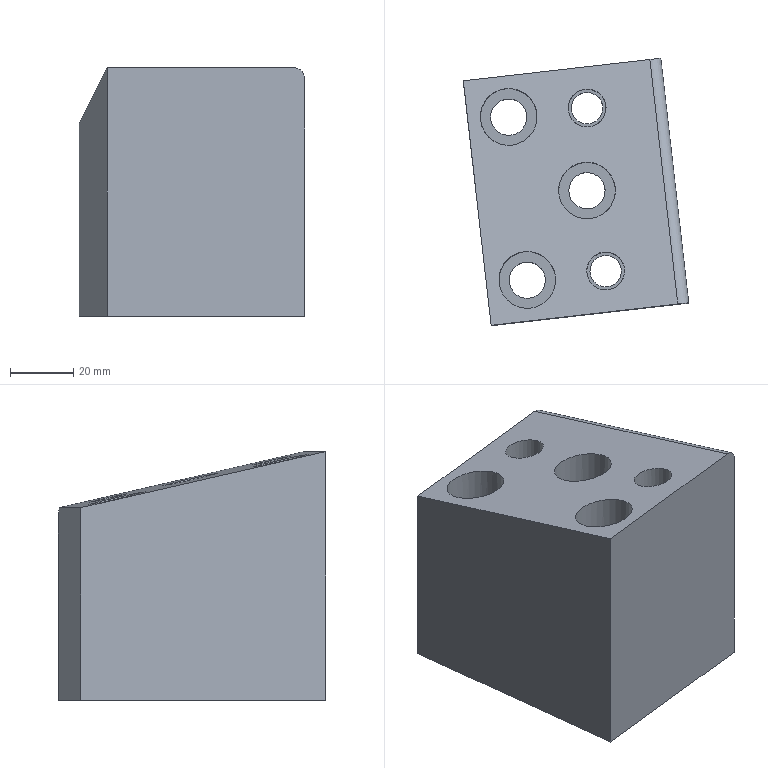Part | NX | features 23 2 | 1 solid | 22 faces | box 71.425 x 84.63 x 78.868 mm | volume 289986 mm3 | plane 11 | cylinder 11 | commonest cylinder face diameters 11.5 x3 18 x3 10.001 x2 12 x2 7 x1
STEP:
#1=CARTESIAN_POINT('',(3732.12,240.405,-83.));
#2=VERTEX_POINT('',#1);
#3=CARTESIAN_POINT('',(3726.517,239.111,-83.));
#4=DIRECTION('',(0.,0.,1.));
#5=DIRECTION('',(0.9744,0.225,0.));
#6=AXIS2_PLACEMENT_3D('',#3,#4,#5);
#7=CIRCLE('',#6,5.75);
#8=EDGE_CURVE('',#2,#2,#7,.T.);
#9=ORIENTED_EDGE('',*,*,#8,.F.);
#10=EDGE_LOOP('',(#9));
#11=FACE_BOUND('',#10,.T.);
#12=CARTESIAN_POINT('',(3735.286,241.136,-83.));
#13=VERTEX_POINT('',#12);
#14=CARTESIAN_POINT('',(3726.517,239.111,-83.));
#15=DIRECTION('',(0.,0.,1.));
#16=DIRECTION('',(0.9744,0.225,0.));
#17=AXIS2_PLACEMENT_3D('',#14,#15,#16);
#18=CIRCLE('',#17,9.);
#19=EDGE_CURVE('',#13,#13,#18,.T.);
#20=ORIENTED_EDGE('',*,*,#19,.T.);
#21=EDGE_LOOP('',(#20));
#22=FACE_BOUND('',#21,.T.);
#23=CARTESIAN_POINT('',(3726.517,239.111,-83.));
#24=DIRECTION('',(0.,0.,-1.));
#25=DIRECTION('',(-0.9744,-0.225,0.));
#26=AXIS2_PLACEMENT_3D('',#23,#24,#25);
#27=PLANE('',#26);
#28=ADVANCED_FACE('',(#11,#22),#27,.F.);
#29=CARTESIAN_POINT('',(3720.767,239.111,-113.));
#30=VERTEX_POINT('',#29);
#31=CARTESIAN_POINT('',(3726.517,239.111,-113.));
#32=DIRECTION('',(0.,0.,1.));
#33=DIRECTION('',(-1.,0.,0.));
#34=AXIS2_PLACEMENT_3D('',#31,#32,#33);
#35=CIRCLE('',#34,5.75);
#36=EDGE_CURVE('',#30,#30,#35,.T.);
#37=ORIENTED_EDGE('',*,*,#36,.F.);
#38=EDGE_LOOP('',(#37));
#39=FACE_BOUND('',#38,.T.);
#40=ORIENTED_EDGE('',*,*,#8,.T.);
#41=EDGE_LOOP('',(#40));
#42=FACE_BOUND('',#41,.T.);
#43=CARTESIAN_POINT('',(3726.517,239.111,-9.166));
#44=DIRECTION('',(0.,0.,-1.));
#45=DIRECTION('',(-0.9744,-0.225,0.));
#46=AXIS2_PLACEMENT_3D('',#43,#44,#45);
#47=CYLINDRICAL_SURFACE('',#46,5.75);
#48=ADVANCED_FACE('',(#39,#42),#47,.F.);
#49=CARTESIAN_POINT('',(3725.498,248.054,-39.145));
#50=VERTEX_POINT('',#49);
#51=CARTESIAN_POINT('',(3726.517,239.111,-37.094));
#52=DIRECTION('',(-0.02515,0.2207,0.975));
#53=DIRECTION('',(-0.1104,0.9687,-0.2221));
#54=AXIS2_PLACEMENT_3D('',#51,#52,#53);
#55=ELLIPSE('',#54,9.231,9.);
#56=EDGE_CURVE('',#50,#50,#55,.T.);
#57=ORIENTED_EDGE('',*,*,#56,.T.);
#58=EDGE_LOOP('',(#57));
#59=FACE_BOUND('',#58,.T.);
#60=ORIENTED_EDGE('',*,*,#19,.F.);
#61=EDGE_LOOP('',(#60));
#62=FACE_BOUND('',#61,.T.);
#63=CARTESIAN_POINT('',(3726.517,239.111,-34.166));
#64=DIRECTION('',(0.,0.,-1.));
#65=DIRECTION('',(-0.9744,-0.225,0.));
#66=AXIS2_PLACEMENT_3D('',#63,#64,#65);
#67=CYLINDRICAL_SURFACE('',#66,9.);
#68=ADVANCED_FACE('',(#59,#62),#67,.F.);
#69=CARTESIAN_POINT('',(3751.035,268.728,-83.));
#70=VERTEX_POINT('',#69);
#71=CARTESIAN_POINT('',(3745.432,267.435,-83.));
#72=DIRECTION('',(0.,0.,1.));
#73=DIRECTION('',(0.9744,0.225,0.));
#74=AXIS2_PLACEMENT_3D('',#71,#72,#73);
#75=CIRCLE('',#74,5.75);
#76=EDGE_CURVE('',#70,#70,#75,.T.);
#77=ORIENTED_EDGE('',*,*,#76,.F.);
#78=EDGE_LOOP('',(#77));
#79=FACE_BOUND('',#78,.T.);
#80=CARTESIAN_POINT('',(3754.202,269.459,-83.));
#81=VERTEX_POINT('',#80);
#82=CARTESIAN_POINT('',(3745.432,267.435,-83.));
#83=DIRECTION('',(0.,0.,1.));
#84=DIRECTION('',(0.9744,0.225,0.));
#85=AXIS2_PLACEMENT_3D('',#82,#83,#84);
#86=CIRCLE('',#85,9.);
#87=EDGE_CURVE('',#81,#81,#86,.T.);
#88=ORIENTED_EDGE('',*,*,#87,.T.);
#89=EDGE_LOOP('',(#88));
#90=FACE_BOUND('',#89,.T.);
#91=CARTESIAN_POINT('',(3745.416,267.58,-83.));
#92=DIRECTION('',(0.,0.,-1.));
#93=DIRECTION('',(-0.9744,-0.225,0.));
#94=AXIS2_PLACEMENT_3D('',#91,#92,#93);
#95=PLANE('',#94);
#96=ADVANCED_FACE('',(#79,#90),#95,.F.);
#97=CARTESIAN_POINT('',(3756.357,241.942,-84.));
#98=VERTEX_POINT('',#97);
#99=CARTESIAN_POINT('',(3751.356,241.942,-84.));
#100=DIRECTION('',(0.,0.,1.));
#101=DIRECTION('',(1.,0.,0.));
#102=AXIS2_PLACEMENT_3D('',#99,#100,#101);
#103=CIRCLE('',#102,5.);
#104=EDGE_CURVE('',#98,#98,#103,.T.);
#105=ORIENTED_EDGE('',*,*,#104,.F.);
#106=EDGE_LOOP('',(#105));
#107=FACE_BOUND('',#106,.T.);
#108=CARTESIAN_POINT('',(3757.356,241.942,-84.));
#109=VERTEX_POINT('',#108);
#110=CARTESIAN_POINT('',(3751.356,241.942,-84.));
#111=DIRECTION('',(0.,0.,1.));
#112=DIRECTION('',(1.,0.,0.));
#113=AXIS2_PLACEMENT_3D('',#110,#111,#112);
#114=CIRCLE('',#113,6.);
#115=EDGE_CURVE('',#109,#109,#114,.T.);
#116=ORIENTED_EDGE('',*,*,#115,.T.);
#117=EDGE_LOOP('',(#116));
#118=FACE_BOUND('',#117,.T.);
#119=CARTESIAN_POINT('',(3751.34,242.086,-84.));
#120=DIRECTION('',(0.,0.,-1.));
#121=DIRECTION('',(-1.,0.,0.));
#122=AXIS2_PLACEMENT_3D('',#119,#120,#121);
#123=PLANE('',#122);
#124=ADVANCED_FACE('',(#107,#118),#123,.F.);
#125=CARTESIAN_POINT('',(3726.38,290.777,-83.));
#126=VERTEX_POINT('',#125);
#127=CARTESIAN_POINT('',(3720.63,290.777,-83.));
#128=DIRECTION('',(0.,0.,1.));
#129=DIRECTION('',(1.,0.,0.));
#130=AXIS2_PLACEMENT_3D('',#127,#128,#129);
#131=CIRCLE('',#130,5.75);
#132=EDGE_CURVE('',#126,#126,#131,.T.);
#133=ORIENTED_EDGE('',*,*,#132,.F.);
#134=EDGE_LOOP('',(#133));
#135=FACE_BOUND('',#134,.T.);
#136=CARTESIAN_POINT('',(3729.63,290.777,-83.));
#137=VERTEX_POINT('',#136);
#138=CARTESIAN_POINT('',(3720.63,290.777,-83.));
#139=DIRECTION('',(0.,0.,1.));
#140=DIRECTION('',(1.,0.,0.));
#141=AXIS2_PLACEMENT_3D('',#138,#139,#140);
#142=CIRCLE('',#141,9.);
#143=EDGE_CURVE('',#137,#137,#142,.T.);
#144=ORIENTED_EDGE('',*,*,#143,.T.);
#145=EDGE_LOOP('',(#144));
#146=FACE_BOUND('',#145,.T.);
#147=CARTESIAN_POINT('',(3720.63,290.777,-83.));
#148=DIRECTION('',(0.,0.,-1.));
#149=DIRECTION('',(-1.,0.,0.));
#150=AXIS2_PLACEMENT_3D('',#147,#148,#149);
#151=PLANE('',#150);
#152=ADVANCED_FACE('',(#135,#146),#151,.F.);
#153=CARTESIAN_POINT('',(3750.342,294.732,-84.));
#154=VERTEX_POINT('',#153);
#155=CARTESIAN_POINT('',(3745.47,293.607,-84.));
#156=DIRECTION('',(0.,0.,1.));
#157=DIRECTION('',(0.9744,0.225,0.));
#158=AXIS2_PLACEMENT_3D('',#155,#156,#157);
#159=CIRCLE('',#158,5.);
#160=EDGE_CURVE('',#154,#154,#159,.T.);
#161=ORIENTED_EDGE('',*,*,#160,.F.);
#162=EDGE_LOOP('',(#161));
#163=FACE_BOUND('',#162,.T.);
#164=CARTESIAN_POINT('',(3751.316,294.957,-84.));
#165=VERTEX_POINT('',#164);
#166=CARTESIAN_POINT('',(3745.47,293.607,-84.));
#167=DIRECTION('',(0.,0.,1.));
#168=DIRECTION('',(0.9744,0.225,0.));
#169=AXIS2_PLACEMENT_3D('',#166,#167,#168);
#170=CIRCLE('',#169,6.);
#171=EDGE_CURVE('',#165,#165,#170,.T.);
#172=ORIENTED_EDGE('',*,*,#171,.T.);
#173=EDGE_LOOP('',(#172));
#174=FACE_BOUND('',#173,.T.);
#175=CARTESIAN_POINT('',(3745.47,293.607,-84.));
#176=DIRECTION('',(0.,0.,-1.));
#177=DIRECTION('',(-0.9744,-0.225,0.));
#178=AXIS2_PLACEMENT_3D('',#175,#176,#177);
#179=PLANE('',#178);
#180=ADVANCED_FACE('',(#163,#174),#179,.F.);
#181=CARTESIAN_POINT('',(3777.667,231.855,-113.));
#182=VERTEX_POINT('',#181);
#183=CARTESIAN_POINT('',(3768.837,309.354,-113.));
#184=VERTEX_POINT('',#183);
#185=CARTESIAN_POINT('',(3797.527,57.547,-113.));
#186=DIRECTION('',(-0.1132,0.9936,0.));
#187=VECTOR('',#186,1000.);
#188=LINE('',#185,#187);
#189=EDGE_CURVE('',#182,#184,#188,.T.);
#190=ORIENTED_EDGE('',*,*,#189,.T.);
#191=CARTESIAN_POINT('',(3768.837,309.354,-55.492));
#192=VERTEX_POINT('',#191);
#193=CARTESIAN_POINT('',(3768.837,309.354,-706.6));
#194=DIRECTION('',(0.000000001,0.,-1.));
#195=VECTOR('',#194,1000.);
#196=LINE('',#193,#195);
#197=EDGE_CURVE('',#192,#184,#196,.T.);
#198=ORIENTED_EDGE('',*,*,#197,.F.);
#199=CARTESIAN_POINT('',(3777.667,231.855,-37.722));
#200=VERTEX_POINT('',#199);
#201=CARTESIAN_POINT('',(3769.383,304.563,-54.394));
#202=DIRECTION('',(0.1104,-0.9687,0.2221));
#203=VECTOR('',#202,1000.);
#204=LINE('',#201,#203);
#205=EDGE_CURVE('',#192,#200,#204,.T.);
#206=ORIENTED_EDGE('',*,*,#205,.T.);
#207=CARTESIAN_POINT('',(3777.667,231.855,-0.000000076));
#208=DIRECTION('',(0.000000001,0.,-1.));
#209=VECTOR('',#208,1000.);
#210=LINE('',#207,#209);
#211=EDGE_CURVE('',#200,#182,#210,.T.);
#212=ORIENTED_EDGE('',*,*,#211,.T.);
#213=EDGE_LOOP('',(#190,#198,#206,#212));
#214=FACE_BOUND('',#213,.T.);
#215=CARTESIAN_POINT('',(3626.296,1560.421,-706.6));
#216=DIRECTION('',(0.9936,0.1132,0.000000001));
#217=DIRECTION('',(0.000000001,-0.000000001,-1.));
#218=AXIS2_PLACEMENT_3D('',#215,#216,#217);
#219=PLANE('',#218);
#220=ADVANCED_FACE('',(#214),#219,.T.);
#221=CARTESIAN_POINT('',(3706.242,302.222,-113.));
#222=VERTEX_POINT('',#221);
#223=CARTESIAN_POINT('',(3706.242,302.222,-51.903));
#224=VERTEX_POINT('',#223);
#225=CARTESIAN_POINT('',(3706.242,302.222,-100.995));
#226=DIRECTION('',(-0.000000001,0.,1.));
#227=VECTOR('',#226,1000.);
#228=LINE('',#225,#227);
#229=EDGE_CURVE('',#222,#224,#228,.T.);
#230=ORIENTED_EDGE('',*,*,#229,.F.);
#231=CARTESIAN_POINT('',(3715.072,224.723,-113.));
#232=VERTEX_POINT('',#231);
#233=CARTESIAN_POINT('',(3734.932,50.416,-113.));
#234=DIRECTION('',(-0.1132,0.9936,0.));
#235=VECTOR('',#234,1000.);
#236=LINE('',#233,#235);
#237=EDGE_CURVE('',#232,#222,#236,.T.);
#238=ORIENTED_EDGE('',*,*,#237,.F.);
#239=CARTESIAN_POINT('',(3715.072,224.723,-34.132));
#240=VERTEX_POINT('',#239);
#241=CARTESIAN_POINT('',(3715.072,224.723,-0.000000121));
#242=DIRECTION('',(0.000000001,0.,-1.));
#243=VECTOR('',#242,1000.);
#244=LINE('',#241,#243);
#245=EDGE_CURVE('',#240,#232,#244,.T.);
#246=ORIENTED_EDGE('',*,*,#245,.F.);
#247=CARTESIAN_POINT('',(3699.139,364.57,-66.199));
#248=DIRECTION('',(-0.1104,0.9687,-0.2221));
#249=VECTOR('',#248,1000.);
#250=LINE('',#247,#249);
#251=EDGE_CURVE('',#240,#224,#250,.T.);
#252=ORIENTED_EDGE('',*,*,#251,.T.);
#253=EDGE_LOOP('',(#230,#238,#246,#252));
#254=FACE_BOUND('',#253,.T.);
#255=CARTESIAN_POINT('',(3563.701,1553.289,-706.6));
#256=DIRECTION('',(0.9936,0.1132,0.000000001));
#257=DIRECTION('',(0.000000001,-0.000000001,-1.));
#258=AXIS2_PLACEMENT_3D('',#255,#256,#257);
#259=PLANE('',#258);
#260=ADVANCED_FACE('',(#254),#259,.F.);
#261=ORIENTED_EDGE('',*,*,#211,.F.);
#262=CARTESIAN_POINT('',(3774.19,231.459,-34.132));
#263=VERTEX_POINT('',#262);
#264=CARTESIAN_POINT('',(3774.19,231.459,-37.722));
#265=DIRECTION('',(0.1132,-0.9936,0.));
#266=DIRECTION('',(-0.000000001,0.,1.));
#267=AXIS2_PLACEMENT_3D('',#264,#265,#266);
#268=ELLIPSE('',#267,3.59,3.5);
#269=EDGE_CURVE('',#200,#263,#268,.T.);
#270=ORIENTED_EDGE('',*,*,#269,.T.);
#271=CARTESIAN_POINT('',(3807.474,235.251,-34.132));
#272=DIRECTION('',(-0.9936,-0.1132,0.000000001));
#273=VECTOR('',#272,1000.);
#274=LINE('',#271,#273);
#275=EDGE_CURVE('',#263,#240,#274,.T.);
#276=ORIENTED_EDGE('',*,*,#275,.T.);
#277=ORIENTED_EDGE('',*,*,#245,.T.);
#278=CARTESIAN_POINT('',(3807.474,235.251,-113.));
#279=DIRECTION('',(-0.9936,-0.1132,0.));
#280=VECTOR('',#279,1000.);
#281=LINE('',#278,#280);
#282=EDGE_CURVE('',#182,#232,#281,.T.);
#283=ORIENTED_EDGE('',*,*,#282,.F.);
#284=EDGE_LOOP('',(#261,#270,#276,#277,#283));
#285=FACE_BOUND('',#284,.T.);
#286=CARTESIAN_POINT('',(3807.474,235.251,-0.000000054));
#287=DIRECTION('',(0.1132,-0.9936,0.));
#288=DIRECTION('',(0.9936,0.1132,0.));
#289=AXIS2_PLACEMENT_3D('',#286,#287,#288);
#290=PLANE('',#289);
#291=ADVANCED_FACE('',(#285),#290,.T.);
#292=CARTESIAN_POINT('',(3765.36,308.958,-51.903));
#293=VERTEX_POINT('',#292);
#294=CARTESIAN_POINT('',(3765.818,304.94,-50.981));
#295=DIRECTION('',(-0.1104,0.9687,-0.2221));
#296=VECTOR('',#295,1000.);
#297=LINE('',#294,#296);
#298=EDGE_CURVE('',#263,#293,#297,.T.);
#299=ORIENTED_EDGE('',*,*,#298,.F.);
#300=ORIENTED_EDGE('',*,*,#269,.F.);
#301=ORIENTED_EDGE('',*,*,#205,.F.);
#302=CARTESIAN_POINT('',(3765.36,308.958,-55.492));
#303=DIRECTION('',(-0.1132,0.9936,0.));
#304=DIRECTION('',(0.,0.,1.));
#305=AXIS2_PLACEMENT_3D('',#302,#303,#304);
#306=ELLIPSE('',#305,3.59,3.5);
#307=EDGE_CURVE('',#293,#192,#306,.T.);
#308=ORIENTED_EDGE('',*,*,#307,.F.);
#309=EDGE_LOOP('',(#299,#300,#301,#308));
#310=FACE_BOUND('',#309,.T.);
#311=CARTESIAN_POINT('',(3768.744,279.254,-48.681));
#312=DIRECTION('',(0.1104,-0.9687,0.2221));
#313=DIRECTION('',(0.6848,0.2361,0.6894));
#314=AXIS2_PLACEMENT_3D('',#311,#312,#313);
#315=CYLINDRICAL_SURFACE('',#314,3.5);
#316=ADVANCED_FACE('',(#310),#315,.T.);
#317=CARTESIAN_POINT('',(1569.81,58.806,-113.));
#318=DIRECTION('',(-0.9936,-0.1132,0.));
#319=VECTOR('',#318,1000.);
#320=LINE('',#317,#319);
#321=EDGE_CURVE('',#184,#222,#320,.T.);
#322=ORIENTED_EDGE('',*,*,#321,.T.);
#323=ORIENTED_EDGE('',*,*,#229,.T.);
#324=CARTESIAN_POINT('',(3772.315,309.75,-51.903));
#325=DIRECTION('',(-0.9936,-0.1132,0.000000001));
#326=VECTOR('',#325,1000.);
#327=LINE('',#324,#326);
#328=EDGE_CURVE('',#293,#224,#327,.T.);
#329=ORIENTED_EDGE('',*,*,#328,.F.);
#330=ORIENTED_EDGE('',*,*,#307,.T.);
#331=ORIENTED_EDGE('',*,*,#197,.T.);
#332=EDGE_LOOP('',(#322,#323,#329,#330,#331));
#333=FACE_BOUND('',#332,.T.);
#334=CARTESIAN_POINT('',(3780.809,310.718,-100.995));
#335=DIRECTION('',(-0.1132,0.9936,0.));
#336=DIRECTION('',(-0.9936,-0.1132,0.));
#337=AXIS2_PLACEMENT_3D('',#334,#335,#336);
#338=PLANE('',#337);
#339=ADVANCED_FACE('',(#333),#338,.T.);
#340=ORIENTED_EDGE('',*,*,#87,.F.);
#341=EDGE_LOOP('',(#340));
#342=FACE_BOUND('',#341,.T.);
#343=CARTESIAN_POINT('',(3744.413,276.377,-45.068));
#344=VERTEX_POINT('',#343);
#345=CARTESIAN_POINT('',(3745.432,267.435,-43.018));
#346=DIRECTION('',(-0.02515,0.2207,0.975));
#347=DIRECTION('',(-0.1104,0.9687,-0.2221));
#348=AXIS2_PLACEMENT_3D('',#345,#346,#347);
#349=ELLIPSE('',#348,9.231,9.);
#350=EDGE_CURVE('',#344,#344,#349,.T.);
#351=ORIENTED_EDGE('',*,*,#350,.T.);
#352=EDGE_LOOP('',(#351));
#353=FACE_BOUND('',#352,.T.);
#354=CARTESIAN_POINT('',(3745.432,267.435,-34.166));
#355=DIRECTION('',(0.,0.,-1.));
#356=DIRECTION('',(-0.9744,-0.225,0.));
#357=AXIS2_PLACEMENT_3D('',#354,#355,#356);
#358=CYLINDRICAL_SURFACE('',#357,9.);
#359=ADVANCED_FACE('',(#342,#353),#358,.F.);
#360=ORIENTED_EDGE('',*,*,#115,.F.);
#361=EDGE_LOOP('',(#360));
#362=FACE_BOUND('',#361,.T.);
#363=CARTESIAN_POINT('',(3750.677,247.903,-38.461));
#364=VERTEX_POINT('',#363);
#365=CARTESIAN_POINT('',(3751.356,241.942,-37.094));
#366=DIRECTION('',(-0.02515,0.2207,0.975));
#367=DIRECTION('',(-0.1104,0.9687,-0.2221));
#368=AXIS2_PLACEMENT_3D('',#365,#366,#367);
#369=ELLIPSE('',#368,6.154,6.);
#370=EDGE_CURVE('',#364,#364,#369,.T.);
#371=ORIENTED_EDGE('',*,*,#370,.T.);
#372=EDGE_LOOP('',(#371));
#373=FACE_BOUND('',#372,.T.);
#374=CARTESIAN_POINT('',(3751.356,241.942,-29.166));
#375=DIRECTION('',(0.,0.,-1.));
#376=DIRECTION('',(-1.,0.,0.));
#377=AXIS2_PLACEMENT_3D('',#374,#375,#376);
#378=CYLINDRICAL_SURFACE('',#377,6.);
#379=ADVANCED_FACE('',(#362,#373),#378,.F.);
#380=ORIENTED_EDGE('',*,*,#143,.F.);
#381=EDGE_LOOP('',(#380));
#382=FACE_BOUND('',#381,.T.);
#383=CARTESIAN_POINT('',(3719.612,299.719,-50.991));
#384=VERTEX_POINT('',#383);
#385=CARTESIAN_POINT('',(3720.63,290.777,-48.941));
#386=DIRECTION('',(-0.02515,0.2207,0.975));
#387=DIRECTION('',(-0.1104,0.9687,-0.2221));
#388=AXIS2_PLACEMENT_3D('',#385,#386,#387);
#389=ELLIPSE('',#388,9.231,9.);
#390=EDGE_CURVE('',#384,#384,#389,.T.);
#391=ORIENTED_EDGE('',*,*,#390,.T.);
#392=EDGE_LOOP('',(#391));
#393=FACE_BOUND('',#392,.T.);
#394=CARTESIAN_POINT('',(3720.63,290.777,-34.166));
#395=DIRECTION('',(0.,0.,-1.));
#396=DIRECTION('',(-1.,0.,0.));
#397=AXIS2_PLACEMENT_3D('',#394,#395,#396);
#398=CYLINDRICAL_SURFACE('',#397,9.);
#399=ADVANCED_FACE('',(#382,#393),#398,.F.);
#400=ORIENTED_EDGE('',*,*,#171,.F.);
#401=EDGE_LOOP('',(#400));
#402=FACE_BOUND('',#401,.T.);
#403=CARTESIAN_POINT('',(3744.79,299.569,-50.308));
#404=VERTEX_POINT('',#403);
#405=CARTESIAN_POINT('',(3745.47,293.607,-48.941));
#406=DIRECTION('',(-0.02515,0.2207,0.975));
#407=DIRECTION('',(-0.1104,0.9687,-0.2221));
#408=AXIS2_PLACEMENT_3D('',#405,#406,#407);
#409=ELLIPSE('',#408,6.154,6.);
#410=EDGE_CURVE('',#404,#404,#409,.T.);
#411=ORIENTED_EDGE('',*,*,#410,.T.);
#412=EDGE_LOOP('',(#411));
#413=FACE_BOUND('',#412,.T.);
#414=CARTESIAN_POINT('',(3745.47,293.607,-29.166));
#415=DIRECTION('',(0.,0.,-1.));
#416=DIRECTION('',(-0.9744,-0.225,0.));
#417=AXIS2_PLACEMENT_3D('',#414,#415,#416);
#418=CYLINDRICAL_SURFACE('',#417,6.);
#419=ADVANCED_FACE('',(#402,#413),#418,.F.);
#420=ORIENTED_EDGE('',*,*,#56,.F.);
#421=EDGE_LOOP('',(#420));
#422=FACE_BOUND('',#421,.T.);
#423=ORIENTED_EDGE('',*,*,#410,.F.);
#424=EDGE_LOOP('',(#423));
#425=FACE_BOUND('',#424,.T.);
#426=ORIENTED_EDGE('',*,*,#390,.F.);
#427=EDGE_LOOP('',(#426));
#428=FACE_BOUND('',#427,.T.);
#429=ORIENTED_EDGE('',*,*,#370,.F.);
#430=EDGE_LOOP('',(#429));
#431=FACE_BOUND('',#430,.T.);
#432=ORIENTED_EDGE('',*,*,#350,.F.);
#433=EDGE_LOOP('',(#432));
#434=FACE_BOUND('',#433,.T.);
#435=ORIENTED_EDGE('',*,*,#328,.T.);
#436=ORIENTED_EDGE('',*,*,#251,.F.);
#437=ORIENTED_EDGE('',*,*,#275,.F.);
#438=ORIENTED_EDGE('',*,*,#298,.T.);
#439=EDGE_LOOP('',(#435,#436,#437,#438));
#440=FACE_BOUND('',#439,.T.);
#441=CARTESIAN_POINT('',(3765.211,372.098,-66.199));
#442=DIRECTION('',(0.02515,-0.2207,-0.975));
#443=DIRECTION('',(-0.1104,0.9687,-0.2221));
#444=AXIS2_PLACEMENT_3D('',#441,#442,#443);
#445=PLANE('',#444);
#446=ADVANCED_FACE('',(#422,#425,#428,#431,#434,#440),#445,.F.);
#447=CARTESIAN_POINT('',(3739.682,267.435,-113.));
#448=VERTEX_POINT('',#447);
#449=CARTESIAN_POINT('',(3745.432,267.435,-113.));
#450=DIRECTION('',(0.,0.,1.));
#451=DIRECTION('',(-1.,0.,0.));
#452=AXIS2_PLACEMENT_3D('',#449,#450,#451);
#453=CIRCLE('',#452,5.75);
#454=EDGE_CURVE('',#448,#448,#453,.T.);
#455=ORIENTED_EDGE('',*,*,#454,.F.);
#456=EDGE_LOOP('',(#455));
#457=FACE_BOUND('',#456,.T.);
#458=ORIENTED_EDGE('',*,*,#76,.T.);
#459=EDGE_LOOP('',(#458));
#460=FACE_BOUND('',#459,.T.);
#461=CARTESIAN_POINT('',(3745.432,267.435,-9.166));
#462=DIRECTION('',(0.,0.,-1.));
#463=DIRECTION('',(-0.9744,-0.225,0.));
#464=AXIS2_PLACEMENT_3D('',#461,#462,#463);
#465=CYLINDRICAL_SURFACE('',#464,5.75);
#466=ADVANCED_FACE('',(#457,#460),#465,.F.);
#467=CARTESIAN_POINT('',(3746.356,241.942,-113.));
#468=VERTEX_POINT('',#467);
#469=CARTESIAN_POINT('',(3751.356,241.942,-113.));
#470=DIRECTION('',(0.,0.,1.));
#471=DIRECTION('',(-1.,0.,0.));
#472=AXIS2_PLACEMENT_3D('',#469,#470,#471);
#473=CIRCLE('',#472,5.);
#474=EDGE_CURVE('',#468,#468,#473,.T.);
#475=ORIENTED_EDGE('',*,*,#474,.F.);
#476=EDGE_LOOP('',(#475));
#477=FACE_BOUND('',#476,.T.);
#478=ORIENTED_EDGE('',*,*,#104,.T.);
#479=EDGE_LOOP('',(#478));
#480=FACE_BOUND('',#479,.T.);
#481=CARTESIAN_POINT('',(3751.356,241.942,-9.166));
#482=DIRECTION('',(0.,0.,-1.));
#483=DIRECTION('',(-1.,0.,0.));
#484=AXIS2_PLACEMENT_3D('',#481,#482,#483);
#485=CYLINDRICAL_SURFACE('',#484,5.);
#486=ADVANCED_FACE('',(#477,#480),#485,.F.);
#487=CARTESIAN_POINT('',(3714.88,290.777,-113.));
#488=VERTEX_POINT('',#487);
#489=CARTESIAN_POINT('',(3720.63,290.777,-113.));
#490=DIRECTION('',(0.,0.,1.));
#491=DIRECTION('',(-1.,0.,0.));
#492=AXIS2_PLACEMENT_3D('',#489,#490,#491);
#493=CIRCLE('',#492,5.75);
#494=EDGE_CURVE('',#488,#488,#493,.T.);
#495=ORIENTED_EDGE('',*,*,#494,.F.);
#496=EDGE_LOOP('',(#495));
#497=FACE_BOUND('',#496,.T.);
#498=ORIENTED_EDGE('',*,*,#132,.T.);
#499=EDGE_LOOP('',(#498));
#500=FACE_BOUND('',#499,.T.);
#501=CARTESIAN_POINT('',(3720.63,290.777,-9.166));
#502=DIRECTION('',(0.,0.,-1.));
#503=DIRECTION('',(-1.,0.,0.));
#504=AXIS2_PLACEMENT_3D('',#501,#502,#503);
#505=CYLINDRICAL_SURFACE('',#504,5.75);
#506=ADVANCED_FACE('',(#497,#500),#505,.F.);
#507=CARTESIAN_POINT('',(3740.469,293.607,-113.));
#508=VERTEX_POINT('',#507);
#509=CARTESIAN_POINT('',(3745.47,293.607,-113.));
#510=DIRECTION('',(0.,0.,1.));
#511=DIRECTION('',(-1.,0.,0.));
#512=AXIS2_PLACEMENT_3D('',#509,#510,#511);
#513=CIRCLE('',#512,5.);
#514=EDGE_CURVE('',#508,#508,#513,.T.);
#515=ORIENTED_EDGE('',*,*,#514,.F.);
#516=EDGE_LOOP('',(#515));
#517=FACE_BOUND('',#516,.T.);
#518=ORIENTED_EDGE('',*,*,#160,.T.);
#519=EDGE_LOOP('',(#518));
#520=FACE_BOUND('',#519,.T.);
#521=CARTESIAN_POINT('',(3745.47,293.607,-9.166));
#522=DIRECTION('',(0.,0.,-1.));
#523=DIRECTION('',(-0.9744,-0.225,0.));
#524=AXIS2_PLACEMENT_3D('',#521,#522,#523);
#525=CYLINDRICAL_SURFACE('',#524,5.);
#526=ADVANCED_FACE('',(#517,#520),#525,.F.);
#527=ORIENTED_EDGE('',*,*,#36,.T.);
#528=EDGE_LOOP('',(#527));
#529=FACE_BOUND('',#528,.T.);
#530=ORIENTED_EDGE('',*,*,#514,.T.);
#531=EDGE_LOOP('',(#530));
#532=FACE_BOUND('',#531,.T.);
#533=ORIENTED_EDGE('',*,*,#494,.T.);
#534=EDGE_LOOP('',(#533));
#535=FACE_BOUND('',#534,.T.);
#536=ORIENTED_EDGE('',*,*,#474,.T.);
#537=EDGE_LOOP('',(#536));
#538=FACE_BOUND('',#537,.T.);
#539=ORIENTED_EDGE('',*,*,#454,.T.);
#540=EDGE_LOOP('',(#539));
#541=FACE_BOUND('',#540,.T.);
#542=ORIENTED_EDGE('',*,*,#282,.T.);
#543=ORIENTED_EDGE('',*,*,#237,.T.);
#544=ORIENTED_EDGE('',*,*,#321,.F.);
#545=ORIENTED_EDGE('',*,*,#189,.F.);
#546=EDGE_LOOP('',(#542,#543,#544,#545));
#547=FACE_BOUND('',#546,.T.);
#548=CARTESIAN_POINT('',(1598.5,-193.,-113.));
#549=DIRECTION('',(0.,0.,-1.));
#550=DIRECTION('',(-1.,0.,0.));
#551=AXIS2_PLACEMENT_3D('',#548,#549,#550);
#552=PLANE('',#551);
#553=ADVANCED_FACE('',(#529,#532,#535,#538,#541,#547),#552,.T.);
#554=CLOSED_SHELL('',(#28,#48,#68,#96,#124,#152,#180,#220,#260,#291,#316,#339,#359,#379,#399,#419,#446,#466,#486,#506,#526,#553));
#555=MANIFOLD_SOLID_BREP('',#554);
#556=(LENGTH_UNIT()NAMED_UNIT(*)SI_UNIT(.MILLI.,.METRE.));
#557=UNCERTAINTY_MEASURE_WITH_UNIT(LENGTH_MEASURE(0.00001),#556,'','');
#558=(NAMED_UNIT(*)PLANE_ANGLE_UNIT()SI_UNIT($,.RADIAN.));
#559=(NAMED_UNIT(*)SI_UNIT($,.STERADIAN.)SOLID_ANGLE_UNIT());
#560=(GEOMETRIC_REPRESENTATION_CONTEXT(3)GLOBAL_UNCERTAINTY_ASSIGNED_CONTEXT((#557))GLOBAL_UNIT_ASSIGNED_CONTEXT((#556,#558,#559))REPRESENTATION_CONTEXT('',''));
#561=ADVANCED_BREP_SHAPE_REPRESENTATION('',(#555),#560);